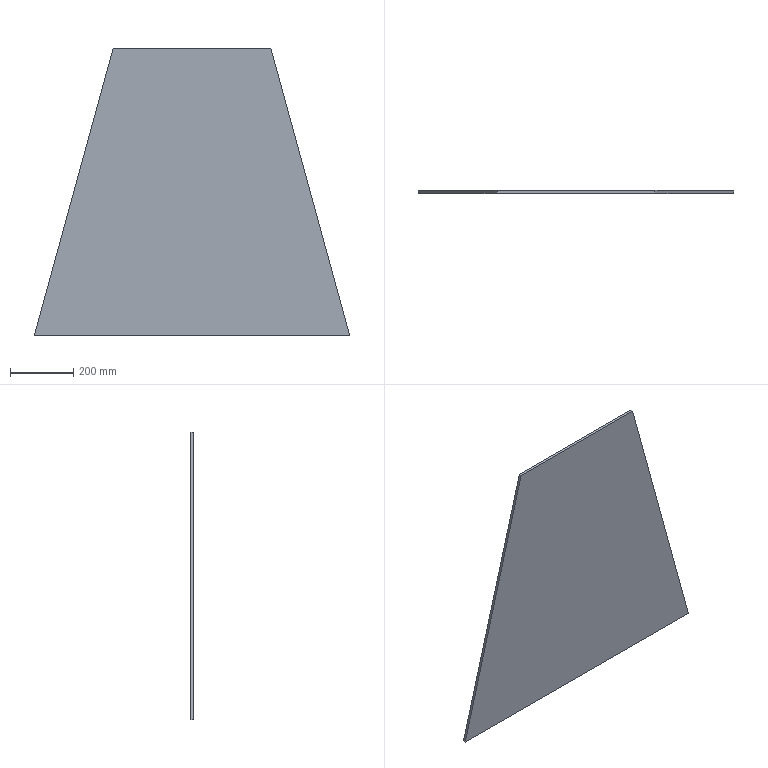Part | SolidWorks | features FlatPattern 1, SMBaseFlange 1, SheetMetal 1 | 1 solid | 6 faces | box 1000 x 8 x 910 mm | volume 5460000 mm3 | plane 6
STEP:
#1=CARTESIAN_POINT('',(0.,0.,0.));
#2=VERTEX_POINT('',#1);
#3=CARTESIAN_POINT('',(250.,0.,910.));
#4=VERTEX_POINT('',#3);
#5=CARTESIAN_POINT('',(250.,0.,910.));
#6=DIRECTION('',(0.2649,0.,0.9643));
#7=VECTOR('',#6,1000.);
#8=LINE('',#5,#7);
#9=EDGE_CURVE('',#2,#4,#8,.T.);
#10=ORIENTED_EDGE('',*,*,#9,.F.);
#11=CARTESIAN_POINT('',(0.,-8.,0.));
#12=VERTEX_POINT('',#11);
#13=CARTESIAN_POINT('',(0.,-8.,0.));
#14=DIRECTION('',(0.,1.,0.));
#15=VECTOR('',#14,1000.);
#16=LINE('',#13,#15);
#17=EDGE_CURVE('',#12,#2,#16,.T.);
#18=ORIENTED_EDGE('',*,*,#17,.F.);
#19=CARTESIAN_POINT('',(250.,-8.,910.));
#20=VERTEX_POINT('',#19);
#21=CARTESIAN_POINT('',(250.,-8.,910.));
#22=DIRECTION('',(0.2649,0.,0.9643));
#23=VECTOR('',#22,1000.);
#24=LINE('',#21,#23);
#25=EDGE_CURVE('',#12,#20,#24,.T.);
#26=ORIENTED_EDGE('',*,*,#25,.T.);
#27=CARTESIAN_POINT('',(250.,-8.,910.));
#28=DIRECTION('',(0.,1.,0.));
#29=VECTOR('',#28,1000.);
#30=LINE('',#27,#29);
#31=EDGE_CURVE('',#20,#4,#30,.T.);
#32=ORIENTED_EDGE('',*,*,#31,.T.);
#33=EDGE_LOOP('',(#10,#18,#26,#32));
#34=FACE_OUTER_BOUND('',#33,.T.);
#35=CARTESIAN_POINT('',(250.,-8.,910.));
#36=DIRECTION('',(-0.9643,0.,0.2649));
#37=DIRECTION('',(0.2649,0.,0.9643));
#38=AXIS2_PLACEMENT_3D('',#35,#36,#37);
#39=PLANE('',#38);
#40=ADVANCED_FACE('',(#34),#39,.T.);
#41=CARTESIAN_POINT('',(1000.,0.,0.));
#42=VERTEX_POINT('',#41);
#43=CARTESIAN_POINT('',(0.,0.,0.));
#44=DIRECTION('',(-1.,0.,0.));
#45=VECTOR('',#44,1000.);
#46=LINE('',#43,#45);
#47=EDGE_CURVE('',#42,#2,#46,.T.);
#48=ORIENTED_EDGE('',*,*,#47,.F.);
#49=CARTESIAN_POINT('',(1000.,-8.,0.));
#50=VERTEX_POINT('',#49);
#51=CARTESIAN_POINT('',(1000.,-8.,0.));
#52=DIRECTION('',(0.,1.,0.));
#53=VECTOR('',#52,1000.);
#54=LINE('',#51,#53);
#55=EDGE_CURVE('',#50,#42,#54,.T.);
#56=ORIENTED_EDGE('',*,*,#55,.F.);
#57=CARTESIAN_POINT('',(0.,-8.,0.));
#58=DIRECTION('',(-1.,0.,0.));
#59=VECTOR('',#58,1000.);
#60=LINE('',#57,#59);
#61=EDGE_CURVE('',#50,#12,#60,.T.);
#62=ORIENTED_EDGE('',*,*,#61,.T.);
#63=ORIENTED_EDGE('',*,*,#17,.T.);
#64=EDGE_LOOP('',(#48,#56,#62,#63));
#65=FACE_OUTER_BOUND('',#64,.T.);
#66=CARTESIAN_POINT('',(0.,-8.,0.));
#67=DIRECTION('',(0.,0.,-1.));
#68=DIRECTION('',(-1.,0.,0.));
#69=AXIS2_PLACEMENT_3D('',#66,#67,#68);
#70=PLANE('',#69);
#71=ADVANCED_FACE('',(#65),#70,.T.);
#72=CARTESIAN_POINT('',(750.,0.,910.));
#73=VERTEX_POINT('',#72);
#74=CARTESIAN_POINT('',(1000.,0.,0.));
#75=DIRECTION('',(0.2649,0.,-0.9643));
#76=VECTOR('',#75,1000.);
#77=LINE('',#74,#76);
#78=EDGE_CURVE('',#73,#42,#77,.T.);
#79=ORIENTED_EDGE('',*,*,#78,.F.);
#80=CARTESIAN_POINT('',(750.,-8.,910.));
#81=VERTEX_POINT('',#80);
#82=CARTESIAN_POINT('',(750.,-8.,910.));
#83=DIRECTION('',(0.,1.,0.));
#84=VECTOR('',#83,1000.);
#85=LINE('',#82,#84);
#86=EDGE_CURVE('',#81,#73,#85,.T.);
#87=ORIENTED_EDGE('',*,*,#86,.F.);
#88=CARTESIAN_POINT('',(1000.,-8.,0.));
#89=DIRECTION('',(0.2649,0.,-0.9643));
#90=VECTOR('',#89,1000.);
#91=LINE('',#88,#90);
#92=EDGE_CURVE('',#81,#50,#91,.T.);
#93=ORIENTED_EDGE('',*,*,#92,.T.);
#94=ORIENTED_EDGE('',*,*,#55,.T.);
#95=EDGE_LOOP('',(#79,#87,#93,#94));
#96=FACE_OUTER_BOUND('',#95,.T.);
#97=CARTESIAN_POINT('',(1000.,-8.,0.));
#98=DIRECTION('',(0.9643,0.,0.2649));
#99=DIRECTION('',(0.2649,0.,-0.9643));
#100=AXIS2_PLACEMENT_3D('',#97,#98,#99);
#101=PLANE('',#100);
#102=ADVANCED_FACE('',(#96),#101,.T.);
#103=CARTESIAN_POINT('',(750.,0.,910.));
#104=DIRECTION('',(1.,0.,0.));
#105=VECTOR('',#104,1000.);
#106=LINE('',#103,#105);
#107=EDGE_CURVE('',#4,#73,#106,.T.);
#108=ORIENTED_EDGE('',*,*,#107,.F.);
#109=ORIENTED_EDGE('',*,*,#31,.F.);
#110=CARTESIAN_POINT('',(750.,-8.,910.));
#111=DIRECTION('',(1.,0.,0.));
#112=VECTOR('',#111,1000.);
#113=LINE('',#110,#112);
#114=EDGE_CURVE('',#20,#81,#113,.T.);
#115=ORIENTED_EDGE('',*,*,#114,.T.);
#116=ORIENTED_EDGE('',*,*,#86,.T.);
#117=EDGE_LOOP('',(#108,#109,#115,#116));
#118=FACE_OUTER_BOUND('',#117,.T.);
#119=CARTESIAN_POINT('',(750.,-8.,910.));
#120=DIRECTION('',(0.,0.,1.));
#121=DIRECTION('',(1.,0.,0.));
#122=AXIS2_PLACEMENT_3D('',#119,#120,#121);
#123=PLANE('',#122);
#124=ADVANCED_FACE('',(#118),#123,.T.);
#125=ORIENTED_EDGE('',*,*,#25,.F.);
#126=ORIENTED_EDGE('',*,*,#61,.F.);
#127=ORIENTED_EDGE('',*,*,#92,.F.);
#128=ORIENTED_EDGE('',*,*,#114,.F.);
#129=EDGE_LOOP('',(#125,#126,#127,#128));
#130=FACE_OUTER_BOUND('',#129,.T.);
#131=CARTESIAN_POINT('',(0.,-8.,0.));
#132=DIRECTION('',(0.,-1.,0.));
#133=DIRECTION('',(0.,0.,-1.));
#134=AXIS2_PLACEMENT_3D('',#131,#132,#133);
#135=PLANE('',#134);
#136=ADVANCED_FACE('',(#130),#135,.T.);
#137=ORIENTED_EDGE('',*,*,#9,.T.);
#138=ORIENTED_EDGE('',*,*,#107,.T.);
#139=ORIENTED_EDGE('',*,*,#78,.T.);
#140=ORIENTED_EDGE('',*,*,#47,.T.);
#141=EDGE_LOOP('',(#137,#138,#139,#140));
#142=FACE_OUTER_BOUND('',#141,.T.);
#143=CARTESIAN_POINT('',(0.,0.,0.));
#144=DIRECTION('',(0.,-1.,0.));
#145=DIRECTION('',(0.,0.,-1.));
#146=AXIS2_PLACEMENT_3D('',#143,#144,#145);
#147=PLANE('',#146);
#148=ADVANCED_FACE('',(#142),#147,.F.);
#149=CLOSED_SHELL('',(#40,#71,#102,#124,#136,#148));
#150=MANIFOLD_SOLID_BREP('',#149);
#151=CARTESIAN_POINT('',(0.,0.,0.));
#152=DIRECTION('',(0.,0.,1.));
#153=DIRECTION('',(1.,0.,0.));
#154=AXIS2_PLACEMENT_3D('',#151,#152,#153);
#155=(LENGTH_UNIT()NAMED_UNIT(*)SI_UNIT(.MILLI.,.METRE.));
#156=UNCERTAINTY_MEASURE_WITH_UNIT(LENGTH_MEASURE(0.00001),#155,'','');
#157=(NAMED_UNIT(*)PLANE_ANGLE_UNIT()SI_UNIT($,.RADIAN.));
#158=(NAMED_UNIT(*)SI_UNIT($,.STERADIAN.)SOLID_ANGLE_UNIT());
#159=(GEOMETRIC_REPRESENTATION_CONTEXT(3)GLOBAL_UNCERTAINTY_ASSIGNED_CONTEXT((#156))GLOBAL_UNIT_ASSIGNED_CONTEXT((#155,#157,#158))REPRESENTATION_CONTEXT('',''));
#160=ADVANCED_BREP_SHAPE_REPRESENTATION('',(#150,#154),#159);